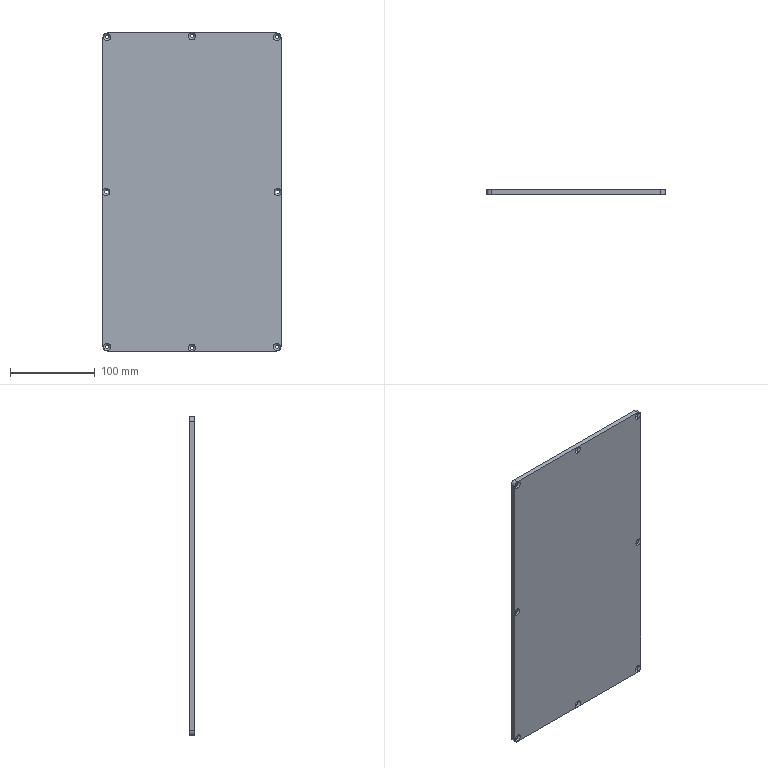Part | SolidWorks | features ICE 42, Fillet 8, DeleteBody 2, Cut 1, Extrusion 1, HoleWzd 1, MoveFace 1, RefAxis 1 | 1 solid | 42 faces | box 210 x 6 x 375 mm | volume 471315 mm3 | cylinder 20 | cone 16 | plane 6 | commonest cylinder face diameters 4.5 x16 10 x4
STEP:
#1=CARTESIAN_POINT('',(196.,-54.,-210.25));
#2=VERTEX_POINT('',#1);
#3=CARTESIAN_POINT('',(196.,-54.,-214.75));
#4=VERTEX_POINT('',#3);
#5=CARTESIAN_POINT('',(196.,-54.,-212.5));
#6=DIRECTION('',(0.,-1.,0.));
#7=DIRECTION('',(0.,0.,-1.));
#8=AXIS2_PLACEMENT_3D('',#5,#6,#7);
#9=CIRCLE('',#8,2.25);
#10=EDGE_CURVE('',#2,#4,#9,.T.);
#11=ORIENTED_EDGE('',*,*,#10,.F.);
#12=CARTESIAN_POINT('',(196.,-56.,-208.25));
#13=VERTEX_POINT('',#12);
#14=CARTESIAN_POINT('',(196.,-56.,-208.25));
#15=DIRECTION('',(0.,-0.7071,0.7071));
#16=VECTOR('',#15,1000.);
#17=LINE('',#14,#16);
#18=EDGE_CURVE('',#2,#13,#17,.T.);
#19=ORIENTED_EDGE('',*,*,#18,.T.);
#20=CARTESIAN_POINT('',(196.,-56.,-216.75));
#21=VERTEX_POINT('',#20);
#22=CARTESIAN_POINT('',(196.,-56.,-212.5));
#23=DIRECTION('',(0.,-1.,0.));
#24=DIRECTION('',(0.,0.,-1.));
#25=AXIS2_PLACEMENT_3D('',#22,#23,#24);
#26=CIRCLE('',#25,4.25);
#27=EDGE_CURVE('',#13,#21,#26,.T.);
#28=ORIENTED_EDGE('',*,*,#27,.T.);
#29=CARTESIAN_POINT('',(196.,-56.,-216.75));
#30=DIRECTION('',(0.,-0.7071,-0.7071));
#31=VECTOR('',#30,1000.);
#32=LINE('',#29,#31);
#33=EDGE_CURVE('',#4,#21,#32,.T.);
#34=ORIENTED_EDGE('',*,*,#33,.F.);
#35=EDGE_LOOP('',(#11,#19,#28,#34));
#36=FACE_OUTER_BOUND('',#35,.T.);
#37=CARTESIAN_POINT('',(196.,-56.,-212.5));
#38=DIRECTION('',(0.,-1.,0.));
#39=DIRECTION('',(0.,0.,-1.));
#40=AXIS2_PLACEMENT_3D('',#37,#38,#39);
#41=CONICAL_SURFACE('',#40,4.25,0.7854);
#42=ADVANCED_FACE('',(#36),#41,.F.);
#43=CARTESIAN_POINT('',(196.,-50.,-210.25));
#44=VERTEX_POINT('',#43);
#45=CARTESIAN_POINT('',(196.,-50.,-214.75));
#46=VERTEX_POINT('',#45);
#47=CARTESIAN_POINT('',(196.,-50.,-212.5));
#48=DIRECTION('',(0.,-1.,0.));
#49=DIRECTION('',(0.,0.,-1.));
#50=AXIS2_PLACEMENT_3D('',#47,#48,#49);
#51=CIRCLE('',#50,2.25);
#52=EDGE_CURVE('',#44,#46,#51,.T.);
#53=ORIENTED_EDGE('',*,*,#52,.F.);
#54=CARTESIAN_POINT('',(196.,-56.,-210.25));
#55=DIRECTION('',(0.,-1.,0.));
#56=VECTOR('',#55,1000.);
#57=LINE('',#54,#56);
#58=EDGE_CURVE('',#44,#2,#57,.T.);
#59=ORIENTED_EDGE('',*,*,#58,.T.);
#60=ORIENTED_EDGE('',*,*,#10,.T.);
#61=CARTESIAN_POINT('',(196.,-56.,-214.75));
#62=DIRECTION('',(0.,-1.,0.));
#63=VECTOR('',#62,1000.);
#64=LINE('',#61,#63);
#65=EDGE_CURVE('',#46,#4,#64,.T.);
#66=ORIENTED_EDGE('',*,*,#65,.F.);
#67=EDGE_LOOP('',(#53,#59,#60,#66));
#68=FACE_OUTER_BOUND('',#67,.T.);
#69=CARTESIAN_POINT('',(196.,-56.,-212.5));
#70=DIRECTION('',(0.,-1.,0.));
#71=DIRECTION('',(0.,0.,-1.));
#72=AXIS2_PLACEMENT_3D('',#69,#70,#71);
#73=CYLINDRICAL_SURFACE('',#72,2.25);
#74=ADVANCED_FACE('',(#68),#73,.F.);
#75=CARTESIAN_POINT('',(195.,-54.,-392.75));
#76=VERTEX_POINT('',#75);
#77=CARTESIAN_POINT('',(195.,-54.,-397.25));
#78=VERTEX_POINT('',#77);
#79=CARTESIAN_POINT('',(195.,-54.,-395.));
#80=DIRECTION('',(0.,-1.,0.));
#81=DIRECTION('',(0.,0.,-1.));
#82=AXIS2_PLACEMENT_3D('',#79,#80,#81);
#83=CIRCLE('',#82,2.25);
#84=EDGE_CURVE('',#76,#78,#83,.T.);
#85=ORIENTED_EDGE('',*,*,#84,.F.);
#86=CARTESIAN_POINT('',(195.,-56.,-390.75));
#87=VERTEX_POINT('',#86);
#88=CARTESIAN_POINT('',(195.,-56.,-390.75));
#89=DIRECTION('',(0.,-0.7071,0.7071));
#90=VECTOR('',#89,1000.);
#91=LINE('',#88,#90);
#92=EDGE_CURVE('',#76,#87,#91,.T.);
#93=ORIENTED_EDGE('',*,*,#92,.T.);
#94=CARTESIAN_POINT('',(195.,-56.,-399.25));
#95=VERTEX_POINT('',#94);
#96=CARTESIAN_POINT('',(195.,-56.,-395.));
#97=DIRECTION('',(0.,-1.,0.));
#98=DIRECTION('',(0.,0.,-1.));
#99=AXIS2_PLACEMENT_3D('',#96,#97,#98);
#100=CIRCLE('',#99,4.25);
#101=EDGE_CURVE('',#87,#95,#100,.T.);
#102=ORIENTED_EDGE('',*,*,#101,.T.);
#103=CARTESIAN_POINT('',(195.,-56.,-399.25));
#104=DIRECTION('',(0.,-0.7071,-0.7071));
#105=VECTOR('',#104,1000.);
#106=LINE('',#103,#105);
#107=EDGE_CURVE('',#78,#95,#106,.T.);
#108=ORIENTED_EDGE('',*,*,#107,.F.);
#109=EDGE_LOOP('',(#85,#93,#102,#108));
#110=FACE_OUTER_BOUND('',#109,.T.);
#111=CARTESIAN_POINT('',(195.,-56.,-395.));
#112=DIRECTION('',(0.,-1.,0.));
#113=DIRECTION('',(0.,0.,-1.));
#114=AXIS2_PLACEMENT_3D('',#111,#112,#113);
#115=CONICAL_SURFACE('',#114,4.25,0.7854);
#116=ADVANCED_FACE('',(#110),#115,.F.);
#117=CARTESIAN_POINT('',(195.,-50.,-392.75));
#118=VERTEX_POINT('',#117);
#119=CARTESIAN_POINT('',(195.,-50.,-397.25));
#120=VERTEX_POINT('',#119);
#121=CARTESIAN_POINT('',(195.,-50.,-395.));
#122=DIRECTION('',(0.,-1.,0.));
#123=DIRECTION('',(0.,0.,-1.));
#124=AXIS2_PLACEMENT_3D('',#121,#122,#123);
#125=CIRCLE('',#124,2.25);
#126=EDGE_CURVE('',#118,#120,#125,.T.);
#127=ORIENTED_EDGE('',*,*,#126,.F.);
#128=CARTESIAN_POINT('',(195.,-56.,-392.75));
#129=DIRECTION('',(0.,-1.,0.));
#130=VECTOR('',#129,1000.);
#131=LINE('',#128,#130);
#132=EDGE_CURVE('',#118,#76,#131,.T.);
#133=ORIENTED_EDGE('',*,*,#132,.T.);
#134=ORIENTED_EDGE('',*,*,#84,.T.);
#135=CARTESIAN_POINT('',(195.,-56.,-397.25));
#136=DIRECTION('',(0.,-1.,0.));
#137=VECTOR('',#136,1000.);
#138=LINE('',#135,#137);
#139=EDGE_CURVE('',#120,#78,#138,.T.);
#140=ORIENTED_EDGE('',*,*,#139,.F.);
#141=EDGE_LOOP('',(#127,#133,#134,#140));
#142=FACE_OUTER_BOUND('',#141,.T.);
#143=CARTESIAN_POINT('',(195.,-56.,-395.));
#144=DIRECTION('',(0.,-1.,0.));
#145=DIRECTION('',(0.,0.,-1.));
#146=AXIS2_PLACEMENT_3D('',#143,#144,#145);
#147=CYLINDRICAL_SURFACE('',#146,2.25);
#148=ADVANCED_FACE('',(#142),#147,.F.);
#149=CARTESIAN_POINT('',(95.,-54.,-393.75));
#150=VERTEX_POINT('',#149);
#151=CARTESIAN_POINT('',(95.,-54.,-398.25));
#152=VERTEX_POINT('',#151);
#153=CARTESIAN_POINT('',(95.,-54.,-396.));
#154=DIRECTION('',(0.,-1.,0.));
#155=DIRECTION('',(0.,0.,-1.));
#156=AXIS2_PLACEMENT_3D('',#153,#154,#155);
#157=CIRCLE('',#156,2.25);
#158=EDGE_CURVE('',#150,#152,#157,.T.);
#159=ORIENTED_EDGE('',*,*,#158,.F.);
#160=CARTESIAN_POINT('',(95.,-56.,-391.75));
#161=VERTEX_POINT('',#160);
#162=CARTESIAN_POINT('',(95.,-56.,-391.75));
#163=DIRECTION('',(0.,-0.7071,0.7071));
#164=VECTOR('',#163,1000.);
#165=LINE('',#162,#164);
#166=EDGE_CURVE('',#150,#161,#165,.T.);
#167=ORIENTED_EDGE('',*,*,#166,.T.);
#168=CARTESIAN_POINT('',(93.564,-56.,-400.));
#169=VERTEX_POINT('',#168);
#170=CARTESIAN_POINT('',(95.,-56.,-396.));
#171=DIRECTION('',(0.,-1.,0.));
#172=DIRECTION('',(0.,0.,-1.));
#173=AXIS2_PLACEMENT_3D('',#170,#171,#172);
#174=CIRCLE('',#173,4.25);
#175=EDGE_CURVE('',#161,#169,#174,.T.);
#176=ORIENTED_EDGE('',*,*,#175,.T.);
#177=CARTESIAN_POINT('',(95.,-55.75,-400.));
#178=VERTEX_POINT('',#177);
#179=CARTESIAN_POINT('',(95.,-55.75,-400.));
#180=CARTESIAN_POINT('',(94.508,-55.75,-400.));
#181=CARTESIAN_POINT('',(94.03,-55.843,-400.));
#182=CARTESIAN_POINT('',(93.564,-56.,-400.));
#183=B_SPLINE_CURVE_WITH_KNOTS('',3,(#179,#180,#181,#182),.UNSPECIFIED.,.F.,.F.,(4,4),(0.02162,0.02307),.UNSPECIFIED.);
#184=EDGE_CURVE('',#178,#169,#183,.T.);
#185=ORIENTED_EDGE('',*,*,#184,.F.);
#186=CARTESIAN_POINT('',(95.,-56.,-400.25));
#187=DIRECTION('',(0.,-0.7071,-0.7071));
#188=VECTOR('',#187,1000.);
#189=LINE('',#186,#188);
#190=EDGE_CURVE('',#152,#178,#189,.T.);
#191=ORIENTED_EDGE('',*,*,#190,.F.);
#192=EDGE_LOOP('',(#159,#167,#176,#185,#191));
#193=FACE_OUTER_BOUND('',#192,.T.);
#194=CARTESIAN_POINT('',(95.,-56.,-396.));
#195=DIRECTION('',(0.,-1.,0.));
#196=DIRECTION('',(0.,0.,-1.));
#197=AXIS2_PLACEMENT_3D('',#194,#195,#196);
#198=CONICAL_SURFACE('',#197,4.25,0.7854);
#199=ADVANCED_FACE('',(#193),#198,.F.);
#200=CARTESIAN_POINT('',(95.,-50.,-393.75));
#201=VERTEX_POINT('',#200);
#202=CARTESIAN_POINT('',(95.,-50.,-398.25));
#203=VERTEX_POINT('',#202);
#204=CARTESIAN_POINT('',(95.,-50.,-396.));
#205=DIRECTION('',(0.,-1.,0.));
#206=DIRECTION('',(0.,0.,-1.));
#207=AXIS2_PLACEMENT_3D('',#204,#205,#206);
#208=CIRCLE('',#207,2.25);
#209=EDGE_CURVE('',#201,#203,#208,.T.);
#210=ORIENTED_EDGE('',*,*,#209,.F.);
#211=CARTESIAN_POINT('',(95.,-56.,-393.75));
#212=DIRECTION('',(0.,-1.,0.));
#213=VECTOR('',#212,1000.);
#214=LINE('',#211,#213);
#215=EDGE_CURVE('',#201,#150,#214,.T.);
#216=ORIENTED_EDGE('',*,*,#215,.T.);
#217=ORIENTED_EDGE('',*,*,#158,.T.);
#218=CARTESIAN_POINT('',(95.,-56.,-398.25));
#219=DIRECTION('',(0.,-1.,0.));
#220=VECTOR('',#219,1000.);
#221=LINE('',#218,#220);
#222=EDGE_CURVE('',#203,#152,#221,.T.);
#223=ORIENTED_EDGE('',*,*,#222,.F.);
#224=EDGE_LOOP('',(#210,#216,#217,#223));
#225=FACE_OUTER_BOUND('',#224,.T.);
#226=CARTESIAN_POINT('',(95.,-56.,-396.));
#227=DIRECTION('',(0.,-1.,0.));
#228=DIRECTION('',(0.,0.,-1.));
#229=AXIS2_PLACEMENT_3D('',#226,#227,#228);
#230=CYLINDRICAL_SURFACE('',#229,2.25);
#231=ADVANCED_FACE('',(#225),#230,.F.);
#232=CARTESIAN_POINT('',(-5.,-54.,-392.75));
#233=VERTEX_POINT('',#232);
#234=CARTESIAN_POINT('',(-5.,-54.,-397.25));
#235=VERTEX_POINT('',#234);
#236=CARTESIAN_POINT('',(-5.,-54.,-395.));
#237=DIRECTION('',(0.,-1.,0.));
#238=DIRECTION('',(0.,0.,-1.));
#239=AXIS2_PLACEMENT_3D('',#236,#237,#238);
#240=CIRCLE('',#239,2.25);
#241=EDGE_CURVE('',#233,#235,#240,.T.);
#242=ORIENTED_EDGE('',*,*,#241,.F.);
#243=CARTESIAN_POINT('',(-5.,-56.,-390.75));
#244=VERTEX_POINT('',#243);
#245=CARTESIAN_POINT('',(-5.,-56.,-390.75));
#246=DIRECTION('',(0.,-0.7071,0.7071));
#247=VECTOR('',#246,1000.);
#248=LINE('',#245,#247);
#249=EDGE_CURVE('',#233,#244,#248,.T.);
#250=ORIENTED_EDGE('',*,*,#249,.T.);
#251=CARTESIAN_POINT('',(-5.,-56.,-399.25));
#252=VERTEX_POINT('',#251);
#253=CARTESIAN_POINT('',(-5.,-56.,-395.));
#254=DIRECTION('',(0.,-1.,0.));
#255=DIRECTION('',(0.,0.,-1.));
#256=AXIS2_PLACEMENT_3D('',#253,#254,#255);
#257=CIRCLE('',#256,4.25);
#258=EDGE_CURVE('',#244,#252,#257,.T.);
#259=ORIENTED_EDGE('',*,*,#258,.T.);
#260=CARTESIAN_POINT('',(-5.,-56.,-399.25));
#261=DIRECTION('',(0.,-0.7071,-0.7071));
#262=VECTOR('',#261,1000.);
#263=LINE('',#260,#262);
#264=EDGE_CURVE('',#235,#252,#263,.T.);
#265=ORIENTED_EDGE('',*,*,#264,.F.);
#266=EDGE_LOOP('',(#242,#250,#259,#265));
#267=FACE_OUTER_BOUND('',#266,.T.);
#268=CARTESIAN_POINT('',(-5.,-56.,-395.));
#269=DIRECTION('',(0.,-1.,0.));
#270=DIRECTION('',(0.,0.,-1.));
#271=AXIS2_PLACEMENT_3D('',#268,#269,#270);
#272=CONICAL_SURFACE('',#271,4.25,0.7854);
#273=ADVANCED_FACE('',(#267),#272,.F.);
#274=CARTESIAN_POINT('',(-5.,-50.,-392.75));
#275=VERTEX_POINT('',#274);
#276=CARTESIAN_POINT('',(-5.,-50.,-397.25));
#277=VERTEX_POINT('',#276);
#278=CARTESIAN_POINT('',(-5.,-50.,-395.));
#279=DIRECTION('',(0.,-1.,0.));
#280=DIRECTION('',(0.,0.,-1.));
#281=AXIS2_PLACEMENT_3D('',#278,#279,#280);
#282=CIRCLE('',#281,2.25);
#283=EDGE_CURVE('',#275,#277,#282,.T.);
#284=ORIENTED_EDGE('',*,*,#283,.F.);
#285=CARTESIAN_POINT('',(-5.,-56.,-392.75));
#286=DIRECTION('',(0.,-1.,0.));
#287=VECTOR('',#286,1000.);
#288=LINE('',#285,#287);
#289=EDGE_CURVE('',#275,#233,#288,.T.);
#290=ORIENTED_EDGE('',*,*,#289,.T.);
#291=ORIENTED_EDGE('',*,*,#241,.T.);
#292=CARTESIAN_POINT('',(-5.,-56.,-397.25));
#293=DIRECTION('',(0.,-1.,0.));
#294=VECTOR('',#293,1000.);
#295=LINE('',#292,#294);
#296=EDGE_CURVE('',#277,#235,#295,.T.);
#297=ORIENTED_EDGE('',*,*,#296,.F.);
#298=EDGE_LOOP('',(#284,#290,#291,#297));
#299=FACE_OUTER_BOUND('',#298,.T.);
#300=CARTESIAN_POINT('',(-5.,-56.,-395.));
#301=DIRECTION('',(0.,-1.,0.));
#302=DIRECTION('',(0.,0.,-1.));
#303=AXIS2_PLACEMENT_3D('',#300,#301,#302);
#304=CYLINDRICAL_SURFACE('',#303,2.25);
#305=ADVANCED_FACE('',(#299),#304,.F.);
#306=CARTESIAN_POINT('',(-6.,-54.,-210.25));
#307=VERTEX_POINT('',#306);
#308=CARTESIAN_POINT('',(-6.,-54.,-214.75));
#309=VERTEX_POINT('',#308);
#310=CARTESIAN_POINT('',(-6.,-54.,-212.5));
#311=DIRECTION('',(0.,-1.,0.));
#312=DIRECTION('',(0.,0.,-1.));
#313=AXIS2_PLACEMENT_3D('',#310,#311,#312);
#314=CIRCLE('',#313,2.25);
#315=EDGE_CURVE('',#307,#309,#314,.T.);
#316=ORIENTED_EDGE('',*,*,#315,.F.);
#317=CARTESIAN_POINT('',(-6.,-56.,-208.25));
#318=VERTEX_POINT('',#317);
#319=CARTESIAN_POINT('',(-6.,-56.,-208.25));
#320=DIRECTION('',(0.,-0.7071,0.7071));
#321=VECTOR('',#320,1000.);
#322=LINE('',#319,#321);
#323=EDGE_CURVE('',#307,#318,#322,.T.);
#324=ORIENTED_EDGE('',*,*,#323,.T.);
#325=CARTESIAN_POINT('',(-10.,-56.,-211.064));
#326=VERTEX_POINT('',#325);
#327=CARTESIAN_POINT('',(-6.,-56.,-212.5));
#328=DIRECTION('',(0.,-1.,0.));
#329=DIRECTION('',(0.,0.,-1.));
#330=AXIS2_PLACEMENT_3D('',#327,#328,#329);
#331=CIRCLE('',#330,4.25);
#332=EDGE_CURVE('',#318,#326,#331,.T.);
#333=ORIENTED_EDGE('',*,*,#332,.T.);
#334=CARTESIAN_POINT('',(-10.,-56.,-213.936));
#335=VERTEX_POINT('',#334);
#336=CARTESIAN_POINT('',(-10.,-56.,-213.936));
#337=CARTESIAN_POINT('',(-10.,-55.843,-213.47));
#338=CARTESIAN_POINT('',(-10.,-55.75,-212.993));
#339=CARTESIAN_POINT('',(-10.,-55.75,-212.255));
#340=CARTESIAN_POINT('',(-10.,-55.773,-212.01));
#341=CARTESIAN_POINT('',(-10.,-55.859,-211.532));
#342=CARTESIAN_POINT('',(-10.,-55.922,-211.296));
#343=CARTESIAN_POINT('',(-10.,-56.,-211.064));
#344=B_SPLINE_CURVE_WITH_KNOTS('',3,(#336,#337,#338,#339,#340,#341,#342,#343),.UNSPECIFIED.,.F.,.F.,(4,2,2,4),(0.01667,0.01812,0.01884,0.01957),.UNSPECIFIED.);
#345=EDGE_CURVE('',#335,#326,#344,.T.);
#346=ORIENTED_EDGE('',*,*,#345,.F.);
#347=CARTESIAN_POINT('',(-6.,-56.,-216.75));
#348=VERTEX_POINT('',#347);
#349=CARTESIAN_POINT('',(-6.,-56.,-212.5));
#350=DIRECTION('',(0.,-1.,0.));
#351=DIRECTION('',(0.,0.,-1.));
#352=AXIS2_PLACEMENT_3D('',#349,#350,#351);
#353=CIRCLE('',#352,4.25);
#354=EDGE_CURVE('',#335,#348,#353,.T.);
#355=ORIENTED_EDGE('',*,*,#354,.T.);
#356=CARTESIAN_POINT('',(-6.,-56.,-216.75));
#357=DIRECTION('',(0.,-0.7071,-0.7071));
#358=VECTOR('',#357,1000.);
#359=LINE('',#356,#358);
#360=EDGE_CURVE('',#309,#348,#359,.T.);
#361=ORIENTED_EDGE('',*,*,#360,.F.);
#362=EDGE_LOOP('',(#316,#324,#333,#346,#355,#361));
#363=FACE_OUTER_BOUND('',#362,.T.);
#364=CARTESIAN_POINT('',(-6.,-56.,-212.5));
#365=DIRECTION('',(0.,-1.,0.));
#366=DIRECTION('',(0.,0.,-1.));
#367=AXIS2_PLACEMENT_3D('',#364,#365,#366);
#368=CONICAL_SURFACE('',#367,4.25,0.7854);
#369=ADVANCED_FACE('',(#363),#368,.F.);
#370=CARTESIAN_POINT('',(-6.,-50.,-210.25));
#371=VERTEX_POINT('',#370);
#372=CARTESIAN_POINT('',(-6.,-50.,-214.75));
#373=VERTEX_POINT('',#372);
#374=CARTESIAN_POINT('',(-6.,-50.,-212.5));
#375=DIRECTION('',(0.,-1.,0.));
#376=DIRECTION('',(0.,0.,-1.));
#377=AXIS2_PLACEMENT_3D('',#374,#375,#376);
#378=CIRCLE('',#377,2.25);
#379=EDGE_CURVE('',#371,#373,#378,.T.);
#380=ORIENTED_EDGE('',*,*,#379,.F.);
#381=CARTESIAN_POINT('',(-6.,-56.,-210.25));
#382=DIRECTION('',(0.,-1.,0.));
#383=VECTOR('',#382,1000.);
#384=LINE('',#381,#383);
#385=EDGE_CURVE('',#371,#307,#384,.T.);
#386=ORIENTED_EDGE('',*,*,#385,.T.);
#387=ORIENTED_EDGE('',*,*,#315,.T.);
#388=CARTESIAN_POINT('',(-6.,-56.,-214.75));
#389=DIRECTION('',(0.,-1.,0.));
#390=VECTOR('',#389,1000.);
#391=LINE('',#388,#390);
#392=EDGE_CURVE('',#373,#309,#391,.T.);
#393=ORIENTED_EDGE('',*,*,#392,.F.);
#394=EDGE_LOOP('',(#380,#386,#387,#393));
#395=FACE_OUTER_BOUND('',#394,.T.);
#396=CARTESIAN_POINT('',(-6.,-56.,-212.5));
#397=DIRECTION('',(0.,-1.,0.));
#398=DIRECTION('',(0.,0.,-1.));
#399=AXIS2_PLACEMENT_3D('',#396,#397,#398);
#400=CYLINDRICAL_SURFACE('',#399,2.25);
#401=ADVANCED_FACE('',(#395),#400,.F.);
#402=CARTESIAN_POINT('',(-5.,-54.,-27.75));
#403=VERTEX_POINT('',#402);
#404=CARTESIAN_POINT('',(-5.,-54.,-32.25));
#405=VERTEX_POINT('',#404);
#406=CARTESIAN_POINT('',(-5.,-54.,-30.));
#407=DIRECTION('',(0.,-1.,0.));
#408=DIRECTION('',(0.,0.,-1.));
#409=AXIS2_PLACEMENT_3D('',#406,#407,#408);
#410=CIRCLE('',#409,2.25);
#411=EDGE_CURVE('',#403,#405,#410,.T.);
#412=ORIENTED_EDGE('',*,*,#411,.F.);
#413=CARTESIAN_POINT('',(-5.,-56.,-25.75));
#414=VERTEX_POINT('',#413);
#415=CARTESIAN_POINT('',(-5.,-56.,-25.75));
#416=DIRECTION('',(0.,-0.7071,0.7071));
#417=VECTOR('',#416,1000.);
#418=LINE('',#415,#417);
#419=EDGE_CURVE('',#403,#414,#418,.T.);
#420=ORIENTED_EDGE('',*,*,#419,.T.);
#421=CARTESIAN_POINT('',(-5.,-56.,-34.25));
#422=VERTEX_POINT('',#421);
#423=CARTESIAN_POINT('',(-5.,-56.,-30.));
#424=DIRECTION('',(0.,-1.,0.));
#425=DIRECTION('',(0.,0.,-1.));
#426=AXIS2_PLACEMENT_3D('',#423,#424,#425);
#427=CIRCLE('',#426,4.25);
#428=EDGE_CURVE('',#414,#422,#427,.T.);
#429=ORIENTED_EDGE('',*,*,#428,.T.);
#430=CARTESIAN_POINT('',(-5.,-56.,-34.25));
#431=DIRECTION('',(0.,-0.7071,-0.7071));
#432=VECTOR('',#431,1000.);
#433=LINE('',#430,#432);
#434=EDGE_CURVE('',#405,#422,#433,.T.);
#435=ORIENTED_EDGE('',*,*,#434,.F.);
#436=EDGE_LOOP('',(#412,#420,#429,#435));
#437=FACE_OUTER_BOUND('',#436,.T.);
#438=CARTESIAN_POINT('',(-5.,-56.,-30.));
#439=DIRECTION('',(0.,-1.,0.));
#440=DIRECTION('',(0.,0.,-1.));
#441=AXIS2_PLACEMENT_3D('',#438,#439,#440);
#442=CONICAL_SURFACE('',#441,4.25,0.7854);
#443=ADVANCED_FACE('',(#437),#442,.F.);
#444=CARTESIAN_POINT('',(-5.,-50.,-27.75));
#445=VERTEX_POINT('',#444);
#446=CARTESIAN_POINT('',(-5.,-50.,-32.25));
#447=VERTEX_POINT('',#446);
#448=CARTESIAN_POINT('',(-5.,-50.,-30.));
#449=DIRECTION('',(0.,-1.,0.));
#450=DIRECTION('',(0.,0.,-1.));
#451=AXIS2_PLACEMENT_3D('',#448,#449,#450);
#452=CIRCLE('',#451,2.25);
#453=EDGE_CURVE('',#445,#447,#452,.T.);
#454=ORIENTED_EDGE('',*,*,#453,.F.);
#455=CARTESIAN_POINT('',(-5.,-56.,-27.75));
#456=DIRECTION('',(0.,-1.,0.));
#457=VECTOR('',#456,1000.);
#458=LINE('',#455,#457);
#459=EDGE_CURVE('',#445,#403,#458,.T.);
#460=ORIENTED_EDGE('',*,*,#459,.T.);
#461=ORIENTED_EDGE('',*,*,#411,.T.);
#462=CARTESIAN_POINT('',(-5.,-56.,-32.25));
#463=DIRECTION('',(0.,-1.,0.));
#464=VECTOR('',#463,1000.);
#465=LINE('',#462,#464);
#466=EDGE_CURVE('',#447,#405,#465,.T.);
#467=ORIENTED_EDGE('',*,*,#466,.F.);
#468=EDGE_LOOP('',(#454,#460,#461,#467));
#469=FACE_OUTER_BOUND('',#468,.T.);
#470=CARTESIAN_POINT('',(-5.,-56.,-30.));
#471=DIRECTION('',(0.,-1.,0.));
#472=DIRECTION('',(0.,0.,-1.));
#473=AXIS2_PLACEMENT_3D('',#470,#471,#472);
#474=CYLINDRICAL_SURFACE('',#473,2.25);
#475=ADVANCED_FACE('',(#469),#474,.F.);
#476=CARTESIAN_POINT('',(95.,-54.,-26.75));
#477=VERTEX_POINT('',#476);
#478=CARTESIAN_POINT('',(95.,-54.,-31.25));
#479=VERTEX_POINT('',#478);
#480=CARTESIAN_POINT('',(95.,-54.,-29.));
#481=DIRECTION('',(0.,-1.,0.));
#482=DIRECTION('',(0.,0.,-1.));
#483=AXIS2_PLACEMENT_3D('',#480,#481,#482);
#484=CIRCLE('',#483,2.25);
#485=EDGE_CURVE('',#477,#479,#484,.T.);
#486=ORIENTED_EDGE('',*,*,#485,.F.);
#487=CARTESIAN_POINT('',(95.,-55.75,-25.));
#488=VERTEX_POINT('',#487);
#489=CARTESIAN_POINT('',(95.,-56.,-24.75));
#490=DIRECTION('',(0.,-0.7071,0.7071));
#491=VECTOR('',#490,1000.);
#492=LINE('',#489,#491);
#493=EDGE_CURVE('',#477,#488,#492,.T.);
#494=ORIENTED_EDGE('',*,*,#493,.T.);
#495=CARTESIAN_POINT('',(93.564,-56.,-25.));
#496=VERTEX_POINT('',#495);
#497=CARTESIAN_POINT('',(93.564,-56.,-25.));
#498=CARTESIAN_POINT('',(94.03,-55.843,-25.));
#499=CARTESIAN_POINT('',(94.508,-55.75,-25.));
#500=CARTESIAN_POINT('',(95.,-55.75,-25.));
#501=B_SPLINE_CURVE_WITH_KNOTS('',3,(#497,#498,#499,#500),.UNSPECIFIED.,.F.,.F.,(4,4),(0.01667,0.01812),.UNSPECIFIED.);
#502=EDGE_CURVE('',#496,#488,#501,.T.);
#503=ORIENTED_EDGE('',*,*,#502,.F.);
#504=CARTESIAN_POINT('',(95.,-56.,-33.25));
#505=VERTEX_POINT('',#504);
#506=CARTESIAN_POINT('',(95.,-56.,-29.));
#507=DIRECTION('',(0.,-1.,0.));
#508=DIRECTION('',(0.,0.,-1.));
#509=AXIS2_PLACEMENT_3D('',#506,#507,#508);
#510=CIRCLE('',#509,4.25);
#511=EDGE_CURVE('',#496,#505,#510,.T.);
#512=ORIENTED_EDGE('',*,*,#511,.T.);
#513=CARTESIAN_POINT('',(95.,-56.,-33.25));
#514=DIRECTION('',(0.,-0.7071,-0.7071));
#515=VECTOR('',#514,1000.);
#516=LINE('',#513,#515);
#517=EDGE_CURVE('',#479,#505,#516,.T.);
#518=ORIENTED_EDGE('',*,*,#517,.F.);
#519=EDGE_LOOP('',(#486,#494,#503,#512,#518));
#520=FACE_OUTER_BOUND('',#519,.T.);
#521=CARTESIAN_POINT('',(95.,-56.,-29.));
#522=DIRECTION('',(0.,-1.,0.));
#523=DIRECTION('',(0.,0.,-1.));
#524=AXIS2_PLACEMENT_3D('',#521,#522,#523);
#525=CONICAL_SURFACE('',#524,4.25,0.7854);
#526=ADVANCED_FACE('',(#520),#525,.F.);
#527=CARTESIAN_POINT('',(95.,-50.,-26.75));
#528=VERTEX_POINT('',#527);
#529=CARTESIAN_POINT('',(95.,-50.,-31.25));
#530=VERTEX_POINT('',#529);
#531=CARTESIAN_POINT('',(95.,-50.,-29.));
#532=DIRECTION('',(0.,-1.,0.));
#533=DIRECTION('',(0.,0.,-1.));
#534=AXIS2_PLACEMENT_3D('',#531,#532,#533);
#535=CIRCLE('',#534,2.25);
#536=EDGE_CURVE('',#528,#530,#535,.T.);
#537=ORIENTED_EDGE('',*,*,#536,.F.);
#538=CARTESIAN_POINT('',(95.,-56.,-26.75));
#539=DIRECTION('',(0.,-1.,0.));
#540=VECTOR('',#539,1000.);
#541=LINE('',#538,#540);
#542=EDGE_CURVE('',#528,#477,#541,.T.);
#543=ORIENTED_EDGE('',*,*,#542,.T.);
#544=ORIENTED_EDGE('',*,*,#485,.T.);
#545=CARTESIAN_POINT('',(95.,-56.,-31.25));
#546=DIRECTION('',(0.,-1.,0.));
#547=VECTOR('',#546,1000.);
#548=LINE('',#545,#547);
#549=EDGE_CURVE('',#530,#479,#548,.T.);
#550=ORIENTED_EDGE('',*,*,#549,.F.);
#551=EDGE_LOOP('',(#537,#543,#544,#550));
#552=FACE_OUTER_BOUND('',#551,.T.);
#553=CARTESIAN_POINT('',(95.,-56.,-29.));
#554=DIRECTION('',(0.,-1.,0.));
#555=DIRECTION('',(0.,0.,-1.));
#556=AXIS2_PLACEMENT_3D('',#553,#554,#555);
#557=CYLINDRICAL_SURFACE('',#556,2.25);
#558=ADVANCED_FACE('',(#552),#557,.F.);
#559=CARTESIAN_POINT('',(195.,-54.,-27.75));
#560=VERTEX_POINT('',#559);
#561=CARTESIAN_POINT('',(195.,-54.,-32.25));
#562=VERTEX_POINT('',#561);
#563=CARTESIAN_POINT('',(195.,-54.,-30.));
#564=DIRECTION('',(0.,-1.,0.));
#565=DIRECTION('',(0.,0.,-1.));
#566=AXIS2_PLACEMENT_3D('',#563,#564,#565);
#567=CIRCLE('',#566,2.25);
#568=EDGE_CURVE('',#560,#562,#567,.T.);
#569=ORIENTED_EDGE('',*,*,#568,.F.);
#570=CARTESIAN_POINT('',(195.,-56.,-25.75));
#571=VERTEX_POINT('',#570);
#572=CARTESIAN_POINT('',(195.,-56.,-25.75));
#573=DIRECTION('',(0.,-0.7071,0.7071));
#574=VECTOR('',#573,1000.);
#575=LINE('',#572,#574);
#576=EDGE_CURVE('',#560,#571,#575,.T.);
#577=ORIENTED_EDGE('',*,*,#576,.T.);
#578=CARTESIAN_POINT('',(195.,-56.,-34.25));
#579=VERTEX_POINT('',#578);
#580=CARTESIAN_POINT('',(195.,-56.,-30.));
#581=DIRECTION('',(0.,-1.,0.));
#582=DIRECTION('',(0.,0.,-1.));
#583=AXIS2_PLACEMENT_3D('',#580,#581,#582);
#584=CIRCLE('',#583,4.25);
#585=EDGE_CURVE('',#571,#579,#584,.T.);
#586=ORIENTED_EDGE('',*,*,#585,.T.);
#587=CARTESIAN_POINT('',(195.,-56.,-34.25));
#588=DIRECTION('',(0.,-0.7071,-0.7071));
#589=VECTOR('',#588,1000.);
#590=LINE('',#587,#589);
#591=EDGE_CURVE('',#562,#579,#590,.T.);
#592=ORIENTED_EDGE('',*,*,#591,.F.);
#593=EDGE_LOOP('',(#569,#577,#586,#592));
#594=FACE_OUTER_BOUND('',#593,.T.);
#595=CARTESIAN_POINT('',(195.,-56.,-30.));
#596=DIRECTION('',(0.,-1.,0.));
#597=DIRECTION('',(0.,0.,-1.));
#598=AXIS2_PLACEMENT_3D('',#595,#596,#597);
#599=CONICAL_SURFACE('',#598,4.25,0.7854);
#600=ADVANCED_FACE('',(#594),#599,.F.);
#601=CARTESIAN_POINT('',(195.,-50.,-27.75));
#602=VERTEX_POINT('',#601);
#603=CARTESIAN_POINT('',(195.,-50.,-32.25));
#604=VERTEX_POINT('',#603);
#605=CARTESIAN_POINT('',(195.,-50.,-30.));
#606=DIRECTION('',(0.,-1.,0.));
#607=DIRECTION('',(0.,0.,-1.));
#608=AXIS2_PLACEMENT_3D('',#605,#606,#607);
#609=CIRCLE('',#608,2.25);
#610=EDGE_CURVE('',#602,#604,#609,.T.);
#611=ORIENTED_EDGE('',*,*,#610,.F.);
#612=CARTESIAN_POINT('',(195.,-56.,-27.75));
#613=DIRECTION('',(0.,-1.,0.));
#614=VECTOR('',#613,1000.);
#615=LINE('',#612,#614);
#616=EDGE_CURVE('',#602,#560,#615,.T.);
#617=ORIENTED_EDGE('',*,*,#616,.T.);
#618=ORIENTED_EDGE('',*,*,#568,.T.);
#619=CARTESIAN_POINT('',(195.,-56.,-32.25));
#620=DIRECTION('',(0.,-1.,0.));
#621=VECTOR('',#620,1000.);
#622=LINE('',#619,#621);
#623=EDGE_CURVE('',#604,#562,#622,.T.);
#624=ORIENTED_EDGE('',*,*,#623,.F.);
#625=EDGE_LOOP('',(#611,#617,#618,#624));
#626=FACE_OUTER_BOUND('',#625,.T.);
#627=CARTESIAN_POINT('',(195.,-56.,-30.));
#628=DIRECTION('',(0.,-1.,0.));
#629=DIRECTION('',(0.,0.,-1.));
#630=AXIS2_PLACEMENT_3D('',#627,#628,#629);
#631=CYLINDRICAL_SURFACE('',#630,2.25);
#632=ADVANCED_FACE('',(#626),#631,.F.);
#633=CARTESIAN_POINT('',(200.,-50.,-30.));
#634=VERTEX_POINT('',#633);
#635=CARTESIAN_POINT('',(195.,-50.,-25.));
#636=VERTEX_POINT('',#635);
#637=CARTESIAN_POINT('',(195.,-50.,-30.));
#638=DIRECTION('',(0.,-1.,0.));
#639=DIRECTION('',(0.,0.,-1.));
#640=AXIS2_PLACEMENT_3D('',#637,#638,#639);
#641=CIRCLE('',#640,5.);
#642=EDGE_CURVE('',#634,#636,#641,.T.);
#643=ORIENTED_EDGE('',*,*,#642,.T.);
#644=CARTESIAN_POINT('',(195.,-56.,-25.));
#645=VERTEX_POINT('',#644);
#646=CARTESIAN_POINT('',(195.,-56.,-25.));
#647=DIRECTION('',(0.,1.,0.));
#648=VECTOR('',#647,1000.);
#649=LINE('',#646,#648);
#650=EDGE_CURVE('',#645,#636,#649,.T.);
#651=ORIENTED_EDGE('',*,*,#650,.F.);
#652=CARTESIAN_POINT('',(200.,-56.,-30.));
#653=VERTEX_POINT('',#652);
#654=CARTESIAN_POINT('',(195.,-56.,-30.));
#655=DIRECTION('',(0.,-1.,0.));
#656=DIRECTION('',(0.,0.,-1.));
#657=AXIS2_PLACEMENT_3D('',#654,#655,#656);
#658=CIRCLE('',#657,5.);
#659=EDGE_CURVE('',#653,#645,#658,.T.);
#660=ORIENTED_EDGE('',*,*,#659,.F.);
#661=CARTESIAN_POINT('',(200.,-56.,-30.));
#662=DIRECTION('',(0.,1.,0.));
#663=VECTOR('',#662,1000.);
#664=LINE('',#661,#663);
#665=EDGE_CURVE('',#653,#634,#664,.T.);
#666=ORIENTED_EDGE('',*,*,#665,.T.);
#667=EDGE_LOOP('',(#643,#651,#660,#666));
#668=FACE_OUTER_BOUND('',#667,.T.);
#669=CARTESIAN_POINT('',(195.,-56.,-30.));
#670=DIRECTION('',(0.,1.,0.));
#671=DIRECTION('',(0.,0.,1.));
#672=AXIS2_PLACEMENT_3D('',#669,#670,#671);
#673=CYLINDRICAL_SURFACE('',#672,5.);
#674=ADVANCED_FACE('',(#668),#673,.T.);
#675=CARTESIAN_POINT('',(-5.,-56.,-25.));
#676=VERTEX_POINT('',#675);
#677=CARTESIAN_POINT('',(195.,-56.,-25.));
#678=DIRECTION('',(-1.,0.,0.));
#679=VECTOR('',#678,1000.);
#680=LINE('',#677,#679);
#681=EDGE_CURVE('',#496,#676,#680,.T.);
#682=ORIENTED_EDGE('',*,*,#681,.F.);
#683=ORIENTED_EDGE('',*,*,#502,.T.);
#684=CARTESIAN_POINT('',(96.436,-56.,-25.));
#685=VERTEX_POINT('',#684);
#686=CARTESIAN_POINT('',(95.,-55.75,-25.));
#687=CARTESIAN_POINT('',(95.246,-55.75,-25.));
#688=CARTESIAN_POINT('',(95.491,-55.773,-25.));
#689=CARTESIAN_POINT('',(95.969,-55.859,-25.));
#690=CARTESIAN_POINT('',(96.204,-55.922,-25.));
#691=CARTESIAN_POINT('',(96.436,-56.,-25.));
#692=B_SPLINE_CURVE_WITH_KNOTS('',3,(#686,#687,#688,#689,#690,#691),.UNSPECIFIED.,.F.,.F.,(4,2,4),(0.01812,0.01884,0.01957),.UNSPECIFIED.);
#693=EDGE_CURVE('',#488,#685,#692,.T.);
#694=ORIENTED_EDGE('',*,*,#693,.T.);
#695=CARTESIAN_POINT('',(195.,-56.,-25.));
#696=DIRECTION('',(-1.,0.,0.));
#697=VECTOR('',#696,1000.);
#698=LINE('',#695,#697);
#699=EDGE_CURVE('',#645,#685,#698,.T.);
#700=ORIENTED_EDGE('',*,*,#699,.F.);
#701=ORIENTED_EDGE('',*,*,#650,.T.);
#702=CARTESIAN_POINT('',(-5.,-50.,-25.));
#703=VERTEX_POINT('',#702);
#704=CARTESIAN_POINT('',(195.,-50.,-25.));
#705=DIRECTION('',(-1.,0.,0.));
#706=VECTOR('',#705,1000.);
#707=LINE('',#704,#706);
#708=EDGE_CURVE('',#636,#703,#707,.T.);
#709=ORIENTED_EDGE('',*,*,#708,.T.);
#710=CARTESIAN_POINT('',(-5.,-56.,-25.));
#711=DIRECTION('',(0.,1.,0.));
#712=VECTOR('',#711,1000.);
#713=LINE('',#710,#712);
#714=EDGE_CURVE('',#676,#703,#713,.T.);
#715=ORIENTED_EDGE('',*,*,#714,.F.);
#716=EDGE_LOOP('',(#682,#683,#694,#700,#701,#709,#715));
#717=FACE_OUTER_BOUND('',#716,.T.);
#718=CARTESIAN_POINT('',(195.,-56.,-25.));
#719=DIRECTION('',(0.,0.,-1.));
#720=DIRECTION('',(-1.,0.,0.));
#721=AXIS2_PLACEMENT_3D('',#718,#719,#720);
#722=PLANE('',#721);
#723=ADVANCED_FACE('',(#717),#722,.F.);
#724=CARTESIAN_POINT('',(-10.,-50.,-30.));
#725=VERTEX_POINT('',#724);
#726=CARTESIAN_POINT('',(-5.,-50.,-30.));
#727=DIRECTION('',(0.,-1.,0.));
#728=DIRECTION('',(0.,0.,-1.));
#729=AXIS2_PLACEMENT_3D('',#726,#727,#728);
#730=CIRCLE('',#729,5.);
#731=EDGE_CURVE('',#703,#725,#730,.T.);
#732=ORIENTED_EDGE('',*,*,#731,.T.);
#733=CARTESIAN_POINT('',(-10.,-56.,-30.));
#734=VERTEX_POINT('',#733);
#735=CARTESIAN_POINT('',(-10.,-56.,-30.));
#736=DIRECTION('',(0.,1.,0.));
#737=VECTOR('',#736,1000.);
#738=LINE('',#735,#737);
#739=EDGE_CURVE('',#734,#725,#738,.T.);
#740=ORIENTED_EDGE('',*,*,#739,.F.);
#741=CARTESIAN_POINT('',(-5.,-56.,-30.));
#742=DIRECTION('',(0.,-1.,0.));
#743=DIRECTION('',(0.,0.,-1.));
#744=AXIS2_PLACEMENT_3D('',#741,#742,#743);
#745=CIRCLE('',#744,5.);
#746=EDGE_CURVE('',#676,#734,#745,.T.);
#747=ORIENTED_EDGE('',*,*,#746,.F.);
#748=ORIENTED_EDGE('',*,*,#714,.T.);
#749=EDGE_LOOP('',(#732,#740,#747,#748));
#750=FACE_OUTER_BOUND('',#749,.T.);
#751=CARTESIAN_POINT('',(-5.,-56.,-30.));
#752=DIRECTION('',(0.,1.,0.));
#753=DIRECTION('',(0.,0.,1.));
#754=AXIS2_PLACEMENT_3D('',#751,#752,#753);
#755=CYLINDRICAL_SURFACE('',#754,5.);
#756=ADVANCED_FACE('',(#750),#755,.T.);
#757=CARTESIAN_POINT('',(-10.,-56.,-395.));
#758=VERTEX_POINT('',#757);
#759=CARTESIAN_POINT('',(-10.,-56.,-30.));
#760=DIRECTION('',(0.,0.,-1.));
#761=VECTOR('',#760,1000.);
#762=LINE('',#759,#761);
#763=EDGE_CURVE('',#335,#758,#762,.T.);
#764=ORIENTED_EDGE('',*,*,#763,.F.);
#765=ORIENTED_EDGE('',*,*,#345,.T.);
#766=CARTESIAN_POINT('',(-10.,-56.,-30.));
#767=DIRECTION('',(0.,0.,-1.));
#768=VECTOR('',#767,1000.);
#769=LINE('',#766,#768);
#770=EDGE_CURVE('',#734,#326,#769,.T.);
#771=ORIENTED_EDGE('',*,*,#770,.F.);
#772=ORIENTED_EDGE('',*,*,#739,.T.);
#773=CARTESIAN_POINT('',(-10.,-50.,-395.));
#774=VERTEX_POINT('',#773);
#775=CARTESIAN_POINT('',(-10.,-50.,-30.));
#776=DIRECTION('',(0.,0.,-1.));
#777=VECTOR('',#776,1000.);
#778=LINE('',#775,#777);
#779=EDGE_CURVE('',#725,#774,#778,.T.);
#780=ORIENTED_EDGE('',*,*,#779,.T.);
#781=CARTESIAN_POINT('',(-10.,-56.,-395.));
#782=DIRECTION('',(0.,1.,0.));
#783=VECTOR('',#782,1000.);
#784=LINE('',#781,#783);
#785=EDGE_CURVE('',#758,#774,#784,.T.);
#786=ORIENTED_EDGE('',*,*,#785,.F.);
#787=EDGE_LOOP('',(#764,#765,#771,#772,#780,#786));
#788=FACE_OUTER_BOUND('',#787,.T.);
#789=CARTESIAN_POINT('',(-10.,-56.,-30.));
#790=DIRECTION('',(1.,0.,0.));
#791=DIRECTION('',(0.,0.,-1.));
#792=AXIS2_PLACEMENT_3D('',#789,#790,#791);
#793=PLANE('',#792);
#794=ADVANCED_FACE('',(#788),#793,.F.);
#795=CARTESIAN_POINT('',(-5.,-50.,-400.));
#796=VERTEX_POINT('',#795);
#797=CARTESIAN_POINT('',(-5.,-50.,-395.));
#798=DIRECTION('',(0.,-1.,0.));
#799=DIRECTION('',(0.,0.,-1.));
#800=AXIS2_PLACEMENT_3D('',#797,#798,#799);
#801=CIRCLE('',#800,5.);
#802=EDGE_CURVE('',#774,#796,#801,.T.);
#803=ORIENTED_EDGE('',*,*,#802,.T.);
#804=CARTESIAN_POINT('',(-5.,-56.,-400.));
#805=VERTEX_POINT('',#804);
#806=CARTESIAN_POINT('',(-5.,-56.,-400.));
#807=DIRECTION('',(0.,1.,0.));
#808=VECTOR('',#807,1000.);
#809=LINE('',#806,#808);
#810=EDGE_CURVE('',#805,#796,#809,.T.);
#811=ORIENTED_EDGE('',*,*,#810,.F.);
#812=CARTESIAN_POINT('',(-5.,-56.,-395.));
#813=DIRECTION('',(0.,-1.,0.));
#814=DIRECTION('',(0.,0.,-1.));
#815=AXIS2_PLACEMENT_3D('',#812,#813,#814);
#816=CIRCLE('',#815,5.);
#817=EDGE_CURVE('',#758,#805,#816,.T.);
#818=ORIENTED_EDGE('',*,*,#817,.F.);
#819=ORIENTED_EDGE('',*,*,#785,.T.);
#820=EDGE_LOOP('',(#803,#811,#818,#819));
#821=FACE_OUTER_BOUND('',#820,.T.);
#822=CARTESIAN_POINT('',(-5.,-56.,-395.));
#823=DIRECTION('',(0.,1.,0.));
#824=DIRECTION('',(0.,0.,1.));
#825=AXIS2_PLACEMENT_3D('',#822,#823,#824);
#826=CYLINDRICAL_SURFACE('',#825,5.);
#827=ADVANCED_FACE('',(#821),#826,.T.);
#828=CARTESIAN_POINT('',(96.436,-56.,-400.));
#829=VERTEX_POINT('',#828);
#830=CARTESIAN_POINT('',(195.,-56.,-400.));
#831=VERTEX_POINT('',#830);
#832=CARTESIAN_POINT('',(-5.,-56.,-400.));
#833=DIRECTION('',(1.,0.,0.));
#834=VECTOR('',#833,1000.);
#835=LINE('',#832,#834);
#836=EDGE_CURVE('',#829,#831,#835,.T.);
#837=ORIENTED_EDGE('',*,*,#836,.F.);
#838=CARTESIAN_POINT('',(96.436,-56.,-400.));
#839=CARTESIAN_POINT('',(96.204,-55.922,-400.));
#840=CARTESIAN_POINT('',(95.969,-55.859,-400.));
#841=CARTESIAN_POINT('',(95.491,-55.773,-400.));
#842=CARTESIAN_POINT('',(95.246,-55.75,-400.));
#843=CARTESIAN_POINT('',(95.,-55.75,-400.));
#844=B_SPLINE_CURVE_WITH_KNOTS('',3,(#838,#839,#840,#841,#842,#843),.UNSPECIFIED.,.F.,.F.,(4,2,4),(0.02017,0.02089,0.02162),.UNSPECIFIED.);
#845=EDGE_CURVE('',#829,#178,#844,.T.);
#846=ORIENTED_EDGE('',*,*,#845,.T.);
#847=ORIENTED_EDGE('',*,*,#184,.T.);
#848=CARTESIAN_POINT('',(-5.,-56.,-400.));
#849=DIRECTION('',(1.,0.,0.));
#850=VECTOR('',#849,1000.);
#851=LINE('',#848,#850);
#852=EDGE_CURVE('',#805,#169,#851,.T.);
#853=ORIENTED_EDGE('',*,*,#852,.F.);
#854=ORIENTED_EDGE('',*,*,#810,.T.);
#855=CARTESIAN_POINT('',(195.,-50.,-400.));
#856=VERTEX_POINT('',#855);
#857=CARTESIAN_POINT('',(-5.,-50.,-400.));
#858=DIRECTION('',(1.,0.,0.));
#859=VECTOR('',#858,1000.);
#860=LINE('',#857,#859);
#861=EDGE_CURVE('',#796,#856,#860,.T.);
#862=ORIENTED_EDGE('',*,*,#861,.T.);
#863=CARTESIAN_POINT('',(195.,-56.,-400.));
#864=DIRECTION('',(0.,1.,0.));
#865=VECTOR('',#864,1000.);
#866=LINE('',#863,#865);
#867=EDGE_CURVE('',#831,#856,#866,.T.);
#868=ORIENTED_EDGE('',*,*,#867,.F.);
#869=EDGE_LOOP('',(#837,#846,#847,#853,#854,#862,#868));
#870=FACE_OUTER_BOUND('',#869,.T.);
#871=CARTESIAN_POINT('',(-5.,-56.,-400.));
#872=DIRECTION('',(0.,0.,1.));
#873=DIRECTION('',(1.,0.,0.));
#874=AXIS2_PLACEMENT_3D('',#871,#872,#873);
#875=PLANE('',#874);
#876=ADVANCED_FACE('',(#870),#875,.F.);
#877=CARTESIAN_POINT('',(200.,-50.,-395.));
#878=VERTEX_POINT('',#877);
#879=CARTESIAN_POINT('',(195.,-50.,-395.));
#880=DIRECTION('',(0.,-1.,0.));
#881=DIRECTION('',(0.,0.,-1.));
#882=AXIS2_PLACEMENT_3D('',#879,#880,#881);
#883=CIRCLE('',#882,5.);
#884=EDGE_CURVE('',#856,#878,#883,.T.);
#885=ORIENTED_EDGE('',*,*,#884,.T.);
#886=CARTESIAN_POINT('',(200.,-56.,-395.));
#887=VERTEX_POINT('',#886);
#888=CARTESIAN_POINT('',(200.,-56.,-395.));
#889=DIRECTION('',(0.,1.,0.));
#890=VECTOR('',#889,1000.);
#891=LINE('',#888,#890);
#892=EDGE_CURVE('',#887,#878,#891,.T.);
#893=ORIENTED_EDGE('',*,*,#892,.F.);
#894=CARTESIAN_POINT('',(195.,-56.,-395.));
#895=DIRECTION('',(0.,-1.,0.));
#896=DIRECTION('',(0.,0.,-1.));
#897=AXIS2_PLACEMENT_3D('',#894,#895,#896);
#898=CIRCLE('',#897,5.);
#899=EDGE_CURVE('',#831,#887,#898,.T.);
#900=ORIENTED_EDGE('',*,*,#899,.F.);
#901=ORIENTED_EDGE('',*,*,#867,.T.);
#902=EDGE_LOOP('',(#885,#893,#900,#901));
#903=FACE_OUTER_BOUND('',#902,.T.);
#904=CARTESIAN_POINT('',(195.,-56.,-395.));
#905=DIRECTION('',(0.,1.,0.));
#906=DIRECTION('',(0.,0.,1.));
#907=AXIS2_PLACEMENT_3D('',#904,#905,#906);
#908=CYLINDRICAL_SURFACE('',#907,5.);
#909=ADVANCED_FACE('',(#903),#908,.T.);
#910=CARTESIAN_POINT('',(200.,-56.,-211.064));
#911=VERTEX_POINT('',#910);
#912=CARTESIAN_POINT('',(200.,-56.,-395.));
#913=DIRECTION('',(0.,0.,1.));
#914=VECTOR('',#913,1000.);
#915=LINE('',#912,#914);
#916=EDGE_CURVE('',#911,#653,#915,.T.);
#917=ORIENTED_EDGE('',*,*,#916,.F.);
#918=CARTESIAN_POINT('',(200.,-56.,-213.936));
#919=VERTEX_POINT('',#918);
#920=CARTESIAN_POINT('',(200.,-56.,-211.064));
#921=CARTESIAN_POINT('',(200.,-55.922,-211.296));
#922=CARTESIAN_POINT('',(200.,-55.859,-211.532));
#923=CARTESIAN_POINT('',(200.,-55.773,-212.01));
#924=CARTESIAN_POINT('',(200.,-55.75,-212.255));
#925=CARTESIAN_POINT('',(200.,-55.75,-212.993));
#926=CARTESIAN_POINT('',(200.,-55.843,-213.47));
#927=CARTESIAN_POINT('',(200.,-56.,-213.936));
#928=B_SPLINE_CURVE_WITH_KNOTS('',3,(#920,#921,#922,#923,#924,#925,#926,#927),.UNSPECIFIED.,.F.,.F.,(4,2,2,4),(0.02017,0.02089,0.02162,0.02307),.UNSPECIFIED.);
#929=EDGE_CURVE('',#911,#919,#928,.T.);
#930=ORIENTED_EDGE('',*,*,#929,.T.);
#931=CARTESIAN_POINT('',(200.,-56.,-395.));
#932=DIRECTION('',(0.,0.,1.));
#933=VECTOR('',#932,1000.);
#934=LINE('',#931,#933);
#935=EDGE_CURVE('',#887,#919,#934,.T.);
#936=ORIENTED_EDGE('',*,*,#935,.F.);
#937=ORIENTED_EDGE('',*,*,#892,.T.);
#938=CARTESIAN_POINT('',(200.,-50.,-395.));
#939=DIRECTION('',(0.,0.,1.));
#940=VECTOR('',#939,1000.);
#941=LINE('',#938,#940);
#942=EDGE_CURVE('',#878,#634,#941,.T.);
#943=ORIENTED_EDGE('',*,*,#942,.T.);
#944=ORIENTED_EDGE('',*,*,#665,.F.);
#945=EDGE_LOOP('',(#917,#930,#936,#937,#943,#944));
#946=FACE_OUTER_BOUND('',#945,.T.);
#947=CARTESIAN_POINT('',(200.,-56.,-395.));
#948=DIRECTION('',(-1.,0.,0.));
#949=DIRECTION('',(0.,0.,1.));
#950=AXIS2_PLACEMENT_3D('',#947,#948,#949);
#951=PLANE('',#950);
#952=ADVANCED_FACE('',(#946),#951,.F.);
#953=CARTESIAN_POINT('',(196.,-56.,-212.5));
#954=DIRECTION('',(0.,-1.,0.));
#955=DIRECTION('',(0.,0.,-1.));
#956=AXIS2_PLACEMENT_3D('',#953,#954,#955);
#957=CIRCLE('',#956,4.25);
#958=EDGE_CURVE('',#911,#13,#957,.T.);
#959=ORIENTED_EDGE('',*,*,#958,.F.);
#960=ORIENTED_EDGE('',*,*,#916,.T.);
#961=ORIENTED_EDGE('',*,*,#659,.T.);
#962=ORIENTED_EDGE('',*,*,#699,.T.);
#963=CARTESIAN_POINT('',(95.,-56.,-29.));
#964=DIRECTION('',(0.,-1.,0.));
#965=DIRECTION('',(0.,0.,-1.));
#966=AXIS2_PLACEMENT_3D('',#963,#964,#965);
#967=CIRCLE('',#966,4.25);
#968=EDGE_CURVE('',#505,#685,#967,.T.);
#969=ORIENTED_EDGE('',*,*,#968,.F.);
#970=ORIENTED_EDGE('',*,*,#511,.F.);
#971=ORIENTED_EDGE('',*,*,#681,.T.);
#972=ORIENTED_EDGE('',*,*,#746,.T.);
#973=ORIENTED_EDGE('',*,*,#770,.T.);
#974=ORIENTED_EDGE('',*,*,#332,.F.);
#975=CARTESIAN_POINT('',(-6.,-56.,-212.5));
#976=DIRECTION('',(0.,-1.,0.));
#977=DIRECTION('',(0.,0.,-1.));
#978=AXIS2_PLACEMENT_3D('',#975,#976,#977);
#979=CIRCLE('',#978,4.25);
#980=EDGE_CURVE('',#348,#318,#979,.T.);
#981=ORIENTED_EDGE('',*,*,#980,.F.);
#982=ORIENTED_EDGE('',*,*,#354,.F.);
#983=ORIENTED_EDGE('',*,*,#763,.T.);
#984=ORIENTED_EDGE('',*,*,#817,.T.);
#985=ORIENTED_EDGE('',*,*,#852,.T.);
#986=ORIENTED_EDGE('',*,*,#175,.F.);
#987=CARTESIAN_POINT('',(95.,-56.,-396.));
#988=DIRECTION('',(0.,-1.,0.));
#989=DIRECTION('',(0.,0.,-1.));
#990=AXIS2_PLACEMENT_3D('',#987,#988,#989);
#991=CIRCLE('',#990,4.25);
#992=EDGE_CURVE('',#829,#161,#991,.T.);
#993=ORIENTED_EDGE('',*,*,#992,.F.);
#994=ORIENTED_EDGE('',*,*,#836,.T.);
#995=ORIENTED_EDGE('',*,*,#899,.T.);
#996=ORIENTED_EDGE('',*,*,#935,.T.);
#997=CARTESIAN_POINT('',(196.,-56.,-212.5));
#998=DIRECTION('',(0.,-1.,0.));
#999=DIRECTION('',(0.,0.,-1.));
#1000=AXIS2_PLACEMENT_3D('',#997,#998,#999);
#1001=CIRCLE('',#1000,4.25);
#1002=EDGE_CURVE('',#21,#919,#1001,.T.);
#1003=ORIENTED_EDGE('',*,*,#1002,.F.);
#1004=ORIENTED_EDGE('',*,*,#27,.F.);
#1005=EDGE_LOOP('',(#959,#960,#961,#962,#969,#970,#971,#972,#973,#974,#981,#982,#983,#984,#985,#986,#993,#994,#995,#996,#1003,#1004));
#1006=FACE_OUTER_BOUND('',#1005,.T.);
#1007=CARTESIAN_POINT('',(195.,-56.,-395.));
#1008=DIRECTION('',(0.,-1.,0.));
#1009=DIRECTION('',(0.,0.,-1.));
#1010=AXIS2_PLACEMENT_3D('',#1007,#1008,#1009);
#1011=CIRCLE('',#1010,4.25);
#1012=EDGE_CURVE('',#95,#87,#1011,.T.);
#1013=ORIENTED_EDGE('',*,*,#1012,.F.);
#1014=ORIENTED_EDGE('',*,*,#101,.F.);
#1015=EDGE_LOOP('',(#1013,#1014));
#1016=FACE_BOUND('',#1015,.T.);
#1017=CARTESIAN_POINT('',(-5.,-56.,-395.));
#1018=DIRECTION('',(0.,-1.,0.));
#1019=DIRECTION('',(0.,0.,-1.));
#1020=AXIS2_PLACEMENT_3D('',#1017,#1018,#1019);
#1021=CIRCLE('',#1020,4.25);
#1022=EDGE_CURVE('',#252,#244,#1021,.T.);
#1023=ORIENTED_EDGE('',*,*,#1022,.F.);
#1024=ORIENTED_EDGE('',*,*,#258,.F.);
#1025=EDGE_LOOP('',(#1023,#1024));
#1026=FACE_BOUND('',#1025,.T.);
#1027=CARTESIAN_POINT('',(-5.,-56.,-30.));
#1028=DIRECTION('',(0.,-1.,0.));
#1029=DIRECTION('',(0.,0.,-1.));
#1030=AXIS2_PLACEMENT_3D('',#1027,#1028,#1029);
#1031=CIRCLE('',#1030,4.25);
#1032=EDGE_CURVE('',#422,#414,#1031,.T.);
#1033=ORIENTED_EDGE('',*,*,#1032,.F.);
#1034=ORIENTED_EDGE('',*,*,#428,.F.);
#1035=EDGE_LOOP('',(#1033,#1034));
#1036=FACE_BOUND('',#1035,.T.);
#1037=CARTESIAN_POINT('',(195.,-56.,-30.));
#1038=DIRECTION('',(0.,-1.,0.));
#1039=DIRECTION('',(0.,0.,-1.));
#1040=AXIS2_PLACEMENT_3D('',#1037,#1038,#1039);
#1041=CIRCLE('',#1040,4.25);
#1042=EDGE_CURVE('',#579,#571,#1041,.T.);
#1043=ORIENTED_EDGE('',*,*,#1042,.F.);
#1044=ORIENTED_EDGE('',*,*,#585,.F.);
#1045=EDGE_LOOP('',(#1043,#1044));
#1046=FACE_BOUND('',#1045,.T.);
#1047=CARTESIAN_POINT('',(195.,-56.,-30.));
#1048=DIRECTION('',(0.,-1.,0.));
#1049=DIRECTION('',(0.,0.,-1.));
#1050=AXIS2_PLACEMENT_3D('',#1047,#1048,#1049);
#1051=PLANE('',#1050);
#1052=ADVANCED_FACE('',(#1006,#1016,#1026,#1036,#1046),#1051,.T.);
#1053=CARTESIAN_POINT('',(196.,-50.,-212.5));
#1054=DIRECTION('',(0.,-1.,0.));
#1055=DIRECTION('',(0.,0.,-1.));
#1056=AXIS2_PLACEMENT_3D('',#1053,#1054,#1055);
#1057=CIRCLE('',#1056,2.25);
#1058=EDGE_CURVE('',#46,#44,#1057,.T.);
#1059=ORIENTED_EDGE('',*,*,#1058,.T.);
#1060=ORIENTED_EDGE('',*,*,#52,.T.);
#1061=EDGE_LOOP('',(#1059,#1060));
#1062=FACE_BOUND('',#1061,.T.);
#1063=CARTESIAN_POINT('',(195.,-50.,-395.));
#1064=DIRECTION('',(0.,-1.,0.));
#1065=DIRECTION('',(0.,0.,-1.));
#1066=AXIS2_PLACEMENT_3D('',#1063,#1064,#1065);
#1067=CIRCLE('',#1066,2.25);
#1068=EDGE_CURVE('',#120,#118,#1067,.T.);
#1069=ORIENTED_EDGE('',*,*,#1068,.T.);
#1070=ORIENTED_EDGE('',*,*,#126,.T.);
#1071=EDGE_LOOP('',(#1069,#1070));
#1072=FACE_BOUND('',#1071,.T.);
#1073=CARTESIAN_POINT('',(95.,-50.,-396.));
#1074=DIRECTION('',(0.,-1.,0.));
#1075=DIRECTION('',(0.,0.,-1.));
#1076=AXIS2_PLACEMENT_3D('',#1073,#1074,#1075);
#1077=CIRCLE('',#1076,2.25);
#1078=EDGE_CURVE('',#203,#201,#1077,.T.);
#1079=ORIENTED_EDGE('',*,*,#1078,.T.);
#1080=ORIENTED_EDGE('',*,*,#209,.T.);
#1081=EDGE_LOOP('',(#1079,#1080));
#1082=FACE_BOUND('',#1081,.T.);
#1083=CARTESIAN_POINT('',(-5.,-50.,-395.));
#1084=DIRECTION('',(0.,-1.,0.));
#1085=DIRECTION('',(0.,0.,-1.));
#1086=AXIS2_PLACEMENT_3D('',#1083,#1084,#1085);
#1087=CIRCLE('',#1086,2.25);
#1088=EDGE_CURVE('',#277,#275,#1087,.T.);
#1089=ORIENTED_EDGE('',*,*,#1088,.T.);
#1090=ORIENTED_EDGE('',*,*,#283,.T.);
#1091=EDGE_LOOP('',(#1089,#1090));
#1092=FACE_BOUND('',#1091,.T.);
#1093=CARTESIAN_POINT('',(-6.,-50.,-212.5));
#1094=DIRECTION('',(0.,-1.,0.));
#1095=DIRECTION('',(0.,0.,-1.));
#1096=AXIS2_PLACEMENT_3D('',#1093,#1094,#1095);
#1097=CIRCLE('',#1096,2.25);
#1098=EDGE_CURVE('',#373,#371,#1097,.T.);
#1099=ORIENTED_EDGE('',*,*,#1098,.T.);
#1100=ORIENTED_EDGE('',*,*,#379,.T.);
#1101=EDGE_LOOP('',(#1099,#1100));
#1102=FACE_BOUND('',#1101,.T.);
#1103=CARTESIAN_POINT('',(-5.,-50.,-30.));
#1104=DIRECTION('',(0.,-1.,0.));
#1105=DIRECTION('',(0.,0.,-1.));
#1106=AXIS2_PLACEMENT_3D('',#1103,#1104,#1105);
#1107=CIRCLE('',#1106,2.25);
#1108=EDGE_CURVE('',#447,#445,#1107,.T.);
#1109=ORIENTED_EDGE('',*,*,#1108,.T.);
#1110=ORIENTED_EDGE('',*,*,#453,.T.);
#1111=EDGE_LOOP('',(#1109,#1110));
#1112=FACE_BOUND('',#1111,.T.);
#1113=CARTESIAN_POINT('',(95.,-50.,-29.));
#1114=DIRECTION('',(0.,-1.,0.));
#1115=DIRECTION('',(0.,0.,-1.));
#1116=AXIS2_PLACEMENT_3D('',#1113,#1114,#1115);
#1117=CIRCLE('',#1116,2.25);
#1118=EDGE_CURVE('',#530,#528,#1117,.T.);
#1119=ORIENTED_EDGE('',*,*,#1118,.T.);
#1120=ORIENTED_EDGE('',*,*,#536,.T.);
#1121=EDGE_LOOP('',(#1119,#1120));
#1122=FACE_BOUND('',#1121,.T.);
#1123=CARTESIAN_POINT('',(195.,-50.,-30.));
#1124=DIRECTION('',(0.,-1.,0.));
#1125=DIRECTION('',(0.,0.,-1.));
#1126=AXIS2_PLACEMENT_3D('',#1123,#1124,#1125);
#1127=CIRCLE('',#1126,2.25);
#1128=EDGE_CURVE('',#604,#602,#1127,.T.);
#1129=ORIENTED_EDGE('',*,*,#1128,.T.);
#1130=ORIENTED_EDGE('',*,*,#610,.T.);
#1131=EDGE_LOOP('',(#1129,#1130));
#1132=FACE_BOUND('',#1131,.T.);
#1133=ORIENTED_EDGE('',*,*,#642,.F.);
#1134=ORIENTED_EDGE('',*,*,#942,.F.);
#1135=ORIENTED_EDGE('',*,*,#884,.F.);
#1136=ORIENTED_EDGE('',*,*,#861,.F.);
#1137=ORIENTED_EDGE('',*,*,#802,.F.);
#1138=ORIENTED_EDGE('',*,*,#779,.F.);
#1139=ORIENTED_EDGE('',*,*,#731,.F.);
#1140=ORIENTED_EDGE('',*,*,#708,.F.);
#1141=EDGE_LOOP('',(#1133,#1134,#1135,#1136,#1137,#1138,#1139,#1140));
#1142=FACE_OUTER_BOUND('',#1141,.T.);
#1143=CARTESIAN_POINT('',(195.,-50.,-30.));
#1144=DIRECTION('',(0.,-1.,0.));
#1145=DIRECTION('',(0.,0.,-1.));
#1146=AXIS2_PLACEMENT_3D('',#1143,#1144,#1145);
#1147=PLANE('',#1146);
#1148=ADVANCED_FACE('',(#1062,#1072,#1082,#1092,#1102,#1112,#1122,#1132,#1142),#1147,.F.);
#1149=ORIENTED_EDGE('',*,*,#616,.F.);
#1150=ORIENTED_EDGE('',*,*,#1128,.F.);
#1151=ORIENTED_EDGE('',*,*,#623,.T.);
#1152=CARTESIAN_POINT('',(195.,-54.,-30.));
#1153=DIRECTION('',(0.,-1.,0.));
#1154=DIRECTION('',(0.,0.,-1.));
#1155=AXIS2_PLACEMENT_3D('',#1152,#1153,#1154);
#1156=CIRCLE('',#1155,2.25);
#1157=EDGE_CURVE('',#562,#560,#1156,.T.);
#1158=ORIENTED_EDGE('',*,*,#1157,.T.);
#1159=EDGE_LOOP('',(#1149,#1150,#1151,#1158));
#1160=FACE_OUTER_BOUND('',#1159,.T.);
#1161=CARTESIAN_POINT('',(195.,-56.,-30.));
#1162=DIRECTION('',(0.,-1.,0.));
#1163=DIRECTION('',(0.,0.,-1.));
#1164=AXIS2_PLACEMENT_3D('',#1161,#1162,#1163);
#1165=CYLINDRICAL_SURFACE('',#1164,2.25);
#1166=ADVANCED_FACE('',(#1160),#1165,.F.);
#1167=ORIENTED_EDGE('',*,*,#576,.F.);
#1168=ORIENTED_EDGE('',*,*,#1157,.F.);
#1169=ORIENTED_EDGE('',*,*,#591,.T.);
#1170=ORIENTED_EDGE('',*,*,#1042,.T.);
#1171=EDGE_LOOP('',(#1167,#1168,#1169,#1170));
#1172=FACE_OUTER_BOUND('',#1171,.T.);
#1173=CARTESIAN_POINT('',(195.,-56.,-30.));
#1174=DIRECTION('',(0.,-1.,0.));
#1175=DIRECTION('',(0.,0.,-1.));
#1176=AXIS2_PLACEMENT_3D('',#1173,#1174,#1175);
#1177=CONICAL_SURFACE('',#1176,4.25,0.7854);
#1178=ADVANCED_FACE('',(#1172),#1177,.F.);
#1179=ORIENTED_EDGE('',*,*,#542,.F.);
#1180=ORIENTED_EDGE('',*,*,#1118,.F.);
#1181=ORIENTED_EDGE('',*,*,#549,.T.);
#1182=CARTESIAN_POINT('',(95.,-54.,-29.));
#1183=DIRECTION('',(0.,-1.,0.));
#1184=DIRECTION('',(0.,0.,-1.));
#1185=AXIS2_PLACEMENT_3D('',#1182,#1183,#1184);
#1186=CIRCLE('',#1185,2.25);
#1187=EDGE_CURVE('',#479,#477,#1186,.T.);
#1188=ORIENTED_EDGE('',*,*,#1187,.T.);
#1189=EDGE_LOOP('',(#1179,#1180,#1181,#1188));
#1190=FACE_OUTER_BOUND('',#1189,.T.);
#1191=CARTESIAN_POINT('',(95.,-56.,-29.));
#1192=DIRECTION('',(0.,-1.,0.));
#1193=DIRECTION('',(0.,0.,-1.));
#1194=AXIS2_PLACEMENT_3D('',#1191,#1192,#1193);
#1195=CYLINDRICAL_SURFACE('',#1194,2.25);
#1196=ADVANCED_FACE('',(#1190),#1195,.F.);
#1197=ORIENTED_EDGE('',*,*,#493,.F.);
#1198=ORIENTED_EDGE('',*,*,#1187,.F.);
#1199=ORIENTED_EDGE('',*,*,#517,.T.);
#1200=ORIENTED_EDGE('',*,*,#968,.T.);
#1201=ORIENTED_EDGE('',*,*,#693,.F.);
#1202=EDGE_LOOP('',(#1197,#1198,#1199,#1200,#1201));
#1203=FACE_OUTER_BOUND('',#1202,.T.);
#1204=CARTESIAN_POINT('',(95.,-56.,-29.));
#1205=DIRECTION('',(0.,-1.,0.));
#1206=DIRECTION('',(0.,0.,-1.));
#1207=AXIS2_PLACEMENT_3D('',#1204,#1205,#1206);
#1208=CONICAL_SURFACE('',#1207,4.25,0.7854);
#1209=ADVANCED_FACE('',(#1203),#1208,.F.);
#1210=ORIENTED_EDGE('',*,*,#459,.F.);
#1211=ORIENTED_EDGE('',*,*,#1108,.F.);
#1212=ORIENTED_EDGE('',*,*,#466,.T.);
#1213=CARTESIAN_POINT('',(-5.,-54.,-30.));
#1214=DIRECTION('',(0.,-1.,0.));
#1215=DIRECTION('',(0.,0.,-1.));
#1216=AXIS2_PLACEMENT_3D('',#1213,#1214,#1215);
#1217=CIRCLE('',#1216,2.25);
#1218=EDGE_CURVE('',#405,#403,#1217,.T.);
#1219=ORIENTED_EDGE('',*,*,#1218,.T.);
#1220=EDGE_LOOP('',(#1210,#1211,#1212,#1219));
#1221=FACE_OUTER_BOUND('',#1220,.T.);
#1222=CARTESIAN_POINT('',(-5.,-56.,-30.));
#1223=DIRECTION('',(0.,-1.,0.));
#1224=DIRECTION('',(0.,0.,-1.));
#1225=AXIS2_PLACEMENT_3D('',#1222,#1223,#1224);
#1226=CYLINDRICAL_SURFACE('',#1225,2.25);
#1227=ADVANCED_FACE('',(#1221),#1226,.F.);
#1228=ORIENTED_EDGE('',*,*,#419,.F.);
#1229=ORIENTED_EDGE('',*,*,#1218,.F.);
#1230=ORIENTED_EDGE('',*,*,#434,.T.);
#1231=ORIENTED_EDGE('',*,*,#1032,.T.);
#1232=EDGE_LOOP('',(#1228,#1229,#1230,#1231));
#1233=FACE_OUTER_BOUND('',#1232,.T.);
#1234=CARTESIAN_POINT('',(-5.,-56.,-30.));
#1235=DIRECTION('',(0.,-1.,0.));
#1236=DIRECTION('',(0.,0.,-1.));
#1237=AXIS2_PLACEMENT_3D('',#1234,#1235,#1236);
#1238=CONICAL_SURFACE('',#1237,4.25,0.7854);
#1239=ADVANCED_FACE('',(#1233),#1238,.F.);
#1240=ORIENTED_EDGE('',*,*,#385,.F.);
#1241=ORIENTED_EDGE('',*,*,#1098,.F.);
#1242=ORIENTED_EDGE('',*,*,#392,.T.);
#1243=CARTESIAN_POINT('',(-6.,-54.,-212.5));
#1244=DIRECTION('',(0.,-1.,0.));
#1245=DIRECTION('',(0.,0.,-1.));
#1246=AXIS2_PLACEMENT_3D('',#1243,#1244,#1245);
#1247=CIRCLE('',#1246,2.25);
#1248=EDGE_CURVE('',#309,#307,#1247,.T.);
#1249=ORIENTED_EDGE('',*,*,#1248,.T.);
#1250=EDGE_LOOP('',(#1240,#1241,#1242,#1249));
#1251=FACE_OUTER_BOUND('',#1250,.T.);
#1252=CARTESIAN_POINT('',(-6.,-56.,-212.5));
#1253=DIRECTION('',(0.,-1.,0.));
#1254=DIRECTION('',(0.,0.,-1.));
#1255=AXIS2_PLACEMENT_3D('',#1252,#1253,#1254);
#1256=CYLINDRICAL_SURFACE('',#1255,2.25);
#1257=ADVANCED_FACE('',(#1251),#1256,.F.);
#1258=ORIENTED_EDGE('',*,*,#323,.F.);
#1259=ORIENTED_EDGE('',*,*,#1248,.F.);
#1260=ORIENTED_EDGE('',*,*,#360,.T.);
#1261=ORIENTED_EDGE('',*,*,#980,.T.);
#1262=EDGE_LOOP('',(#1258,#1259,#1260,#1261));
#1263=FACE_OUTER_BOUND('',#1262,.T.);
#1264=CARTESIAN_POINT('',(-6.,-56.,-212.5));
#1265=DIRECTION('',(0.,-1.,0.));
#1266=DIRECTION('',(0.,0.,-1.));
#1267=AXIS2_PLACEMENT_3D('',#1264,#1265,#1266);
#1268=CONICAL_SURFACE('',#1267,4.25,0.7854);
#1269=ADVANCED_FACE('',(#1263),#1268,.F.);
#1270=ORIENTED_EDGE('',*,*,#289,.F.);
#1271=ORIENTED_EDGE('',*,*,#1088,.F.);
#1272=ORIENTED_EDGE('',*,*,#296,.T.);
#1273=CARTESIAN_POINT('',(-5.,-54.,-395.));
#1274=DIRECTION('',(0.,-1.,0.));
#1275=DIRECTION('',(0.,0.,-1.));
#1276=AXIS2_PLACEMENT_3D('',#1273,#1274,#1275);
#1277=CIRCLE('',#1276,2.25);
#1278=EDGE_CURVE('',#235,#233,#1277,.T.);
#1279=ORIENTED_EDGE('',*,*,#1278,.T.);
#1280=EDGE_LOOP('',(#1270,#1271,#1272,#1279));
#1281=FACE_OUTER_BOUND('',#1280,.T.);
#1282=CARTESIAN_POINT('',(-5.,-56.,-395.));
#1283=DIRECTION('',(0.,-1.,0.));
#1284=DIRECTION('',(0.,0.,-1.));
#1285=AXIS2_PLACEMENT_3D('',#1282,#1283,#1284);
#1286=CYLINDRICAL_SURFACE('',#1285,2.25);
#1287=ADVANCED_FACE('',(#1281),#1286,.F.);
#1288=ORIENTED_EDGE('',*,*,#249,.F.);
#1289=ORIENTED_EDGE('',*,*,#1278,.F.);
#1290=ORIENTED_EDGE('',*,*,#264,.T.);
#1291=ORIENTED_EDGE('',*,*,#1022,.T.);
#1292=EDGE_LOOP('',(#1288,#1289,#1290,#1291));
#1293=FACE_OUTER_BOUND('',#1292,.T.);
#1294=CARTESIAN_POINT('',(-5.,-56.,-395.));
#1295=DIRECTION('',(0.,-1.,0.));
#1296=DIRECTION('',(0.,0.,-1.));
#1297=AXIS2_PLACEMENT_3D('',#1294,#1295,#1296);
#1298=CONICAL_SURFACE('',#1297,4.25,0.7854);
#1299=ADVANCED_FACE('',(#1293),#1298,.F.);
#1300=ORIENTED_EDGE('',*,*,#215,.F.);
#1301=ORIENTED_EDGE('',*,*,#1078,.F.);
#1302=ORIENTED_EDGE('',*,*,#222,.T.);
#1303=CARTESIAN_POINT('',(95.,-54.,-396.));
#1304=DIRECTION('',(0.,-1.,0.));
#1305=DIRECTION('',(0.,0.,-1.));
#1306=AXIS2_PLACEMENT_3D('',#1303,#1304,#1305);
#1307=CIRCLE('',#1306,2.25);
#1308=EDGE_CURVE('',#152,#150,#1307,.T.);
#1309=ORIENTED_EDGE('',*,*,#1308,.T.);
#1310=EDGE_LOOP('',(#1300,#1301,#1302,#1309));
#1311=FACE_OUTER_BOUND('',#1310,.T.);
#1312=CARTESIAN_POINT('',(95.,-56.,-396.));
#1313=DIRECTION('',(0.,-1.,0.));
#1314=DIRECTION('',(0.,0.,-1.));
#1315=AXIS2_PLACEMENT_3D('',#1312,#1313,#1314);
#1316=CYLINDRICAL_SURFACE('',#1315,2.25);
#1317=ADVANCED_FACE('',(#1311),#1316,.F.);
#1318=ORIENTED_EDGE('',*,*,#166,.F.);
#1319=ORIENTED_EDGE('',*,*,#1308,.F.);
#1320=ORIENTED_EDGE('',*,*,#190,.T.);
#1321=ORIENTED_EDGE('',*,*,#845,.F.);
#1322=ORIENTED_EDGE('',*,*,#992,.T.);
#1323=EDGE_LOOP('',(#1318,#1319,#1320,#1321,#1322));
#1324=FACE_OUTER_BOUND('',#1323,.T.);
#1325=CARTESIAN_POINT('',(95.,-56.,-396.));
#1326=DIRECTION('',(0.,-1.,0.));
#1327=DIRECTION('',(0.,0.,-1.));
#1328=AXIS2_PLACEMENT_3D('',#1325,#1326,#1327);
#1329=CONICAL_SURFACE('',#1328,4.25,0.7854);
#1330=ADVANCED_FACE('',(#1324),#1329,.F.);
#1331=ORIENTED_EDGE('',*,*,#132,.F.);
#1332=ORIENTED_EDGE('',*,*,#1068,.F.);
#1333=ORIENTED_EDGE('',*,*,#139,.T.);
#1334=CARTESIAN_POINT('',(195.,-54.,-395.));
#1335=DIRECTION('',(0.,-1.,0.));
#1336=DIRECTION('',(0.,0.,-1.));
#1337=AXIS2_PLACEMENT_3D('',#1334,#1335,#1336);
#1338=CIRCLE('',#1337,2.25);
#1339=EDGE_CURVE('',#78,#76,#1338,.T.);
#1340=ORIENTED_EDGE('',*,*,#1339,.T.);
#1341=EDGE_LOOP('',(#1331,#1332,#1333,#1340));
#1342=FACE_OUTER_BOUND('',#1341,.T.);
#1343=CARTESIAN_POINT('',(195.,-56.,-395.));
#1344=DIRECTION('',(0.,-1.,0.));
#1345=DIRECTION('',(0.,0.,-1.));
#1346=AXIS2_PLACEMENT_3D('',#1343,#1344,#1345);
#1347=CYLINDRICAL_SURFACE('',#1346,2.25);
#1348=ADVANCED_FACE('',(#1342),#1347,.F.);
#1349=ORIENTED_EDGE('',*,*,#92,.F.);
#1350=ORIENTED_EDGE('',*,*,#1339,.F.);
#1351=ORIENTED_EDGE('',*,*,#107,.T.);
#1352=ORIENTED_EDGE('',*,*,#1012,.T.);
#1353=EDGE_LOOP('',(#1349,#1350,#1351,#1352));
#1354=FACE_OUTER_BOUND('',#1353,.T.);
#1355=CARTESIAN_POINT('',(195.,-56.,-395.));
#1356=DIRECTION('',(0.,-1.,0.));
#1357=DIRECTION('',(0.,0.,-1.));
#1358=AXIS2_PLACEMENT_3D('',#1355,#1356,#1357);
#1359=CONICAL_SURFACE('',#1358,4.25,0.7854);
#1360=ADVANCED_FACE('',(#1354),#1359,.F.);
#1361=ORIENTED_EDGE('',*,*,#58,.F.);
#1362=ORIENTED_EDGE('',*,*,#1058,.F.);
#1363=ORIENTED_EDGE('',*,*,#65,.T.);
#1364=CARTESIAN_POINT('',(196.,-54.,-212.5));
#1365=DIRECTION('',(0.,-1.,0.));
#1366=DIRECTION('',(0.,0.,-1.));
#1367=AXIS2_PLACEMENT_3D('',#1364,#1365,#1366);
#1368=CIRCLE('',#1367,2.25);
#1369=EDGE_CURVE('',#4,#2,#1368,.T.);
#1370=ORIENTED_EDGE('',*,*,#1369,.T.);
#1371=EDGE_LOOP('',(#1361,#1362,#1363,#1370));
#1372=FACE_OUTER_BOUND('',#1371,.T.);
#1373=CARTESIAN_POINT('',(196.,-56.,-212.5));
#1374=DIRECTION('',(0.,-1.,0.));
#1375=DIRECTION('',(0.,0.,-1.));
#1376=AXIS2_PLACEMENT_3D('',#1373,#1374,#1375);
#1377=CYLINDRICAL_SURFACE('',#1376,2.25);
#1378=ADVANCED_FACE('',(#1372),#1377,.F.);
#1379=ORIENTED_EDGE('',*,*,#18,.F.);
#1380=ORIENTED_EDGE('',*,*,#1369,.F.);
#1381=ORIENTED_EDGE('',*,*,#33,.T.);
#1382=ORIENTED_EDGE('',*,*,#1002,.T.);
#1383=ORIENTED_EDGE('',*,*,#929,.F.);
#1384=ORIENTED_EDGE('',*,*,#958,.T.);
#1385=EDGE_LOOP('',(#1379,#1380,#1381,#1382,#1383,#1384));
#1386=FACE_OUTER_BOUND('',#1385,.T.);
#1387=CARTESIAN_POINT('',(196.,-56.,-212.5));
#1388=DIRECTION('',(0.,-1.,0.));
#1389=DIRECTION('',(0.,0.,-1.));
#1390=AXIS2_PLACEMENT_3D('',#1387,#1388,#1389);
#1391=CONICAL_SURFACE('',#1390,4.25,0.7854);
#1392=ADVANCED_FACE('',(#1386),#1391,.F.);
#1393=CLOSED_SHELL('',(#42,#74,#116,#148,#199,#231,#273,#305,#369,#401,#443,#475,#526,#558,#600,#632,#674,#723,#756,#794,#827,#876,#909,#952,#1052,#1148,#1166,#1178,#1196,#1209,#1227,#1239,#1257,#1269,#1287,#1299,#1317,#1330,#1348,#1360,#1378,#1392));
#1394=MANIFOLD_SOLID_BREP('',#1393);
#1395=CARTESIAN_POINT('',(0.,0.,0.));
#1396=DIRECTION('',(0.,0.,1.));
#1397=DIRECTION('',(1.,0.,0.));
#1398=AXIS2_PLACEMENT_3D('',#1395,#1396,#1397);
#1399=(LENGTH_UNIT()NAMED_UNIT(*)SI_UNIT(.MILLI.,.METRE.));
#1400=UNCERTAINTY_MEASURE_WITH_UNIT(LENGTH_MEASURE(0.00001),#1399,'','');
#1401=(NAMED_UNIT(*)PLANE_ANGLE_UNIT()SI_UNIT($,.RADIAN.));
#1402=(NAMED_UNIT(*)SI_UNIT($,.STERADIAN.)SOLID_ANGLE_UNIT());
#1403=(GEOMETRIC_REPRESENTATION_CONTEXT(3)GLOBAL_UNCERTAINTY_ASSIGNED_CONTEXT((#1400))GLOBAL_UNIT_ASSIGNED_CONTEXT((#1399,#1401,#1402))REPRESENTATION_CONTEXT('',''));
#1404=ADVANCED_BREP_SHAPE_REPRESENTATION('',(#1394,#1398),#1403);